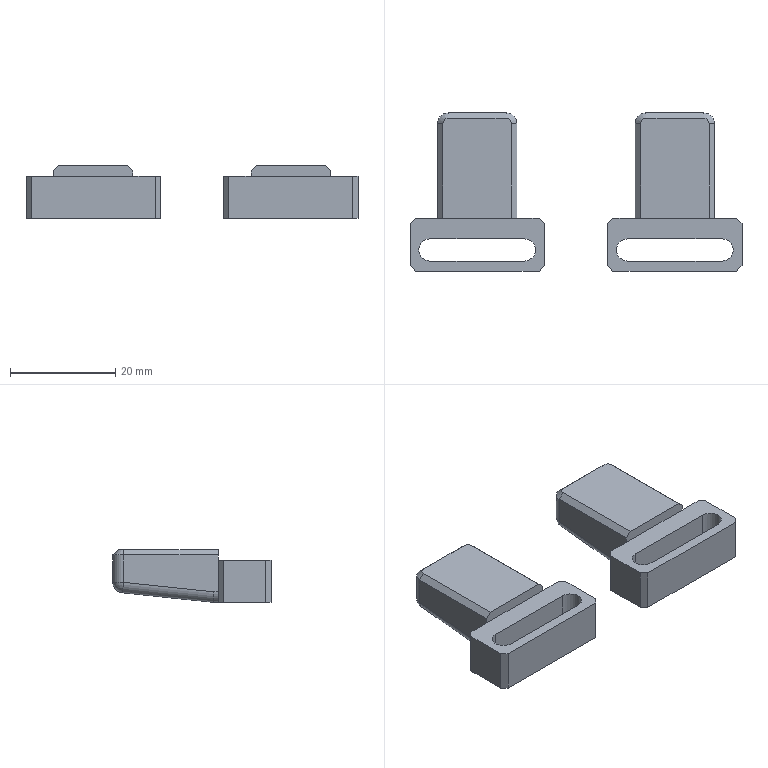NC program | NX | posted with a generic post | part box 63 x 30 x 10 mm
Lines 1 to 136 of 24780:
N10 G17 G21 G94 G90
(FLOOR_WALL_COPY_COPY , TOOL : D80)
N12 T19 M6
N14 G54
N16 G17 G0 G90 X78.5 Y0. B0. C0. S6500 M3
N18 G43 Z30. H19
N20 Z7.04
N22 G94 G1 Z4.04 F1500.
N24 X73.5
N26 X-73.5
N28 X-78.5
N30 Z7.04
N32 G0 Z30.
N34 X78.5
N36 Z6.08
N38 G1 Z3.08
N40 X73.5
N42 X-73.5
N44 X-78.5
N46 Z6.08
N48 G0 Z30.
N50 X78.5
N52 Z5.12
N54 G1 Z2.12
N56 X73.5
N58 X-73.5
N60 X-78.5
N62 Z5.12
N64 G0 Z30.
N66 X78.5
N68 Z4.16
N70 G1 Z1.16
N72 X73.5
N74 X-73.5
N76 X-78.5
N78 Z4.16
N80 G0 Z30.
N82 X78.5
N84 Z3.2
N86 G1 Z0.2
N88 X73.5
N90 X-73.5
N92 X-78.5
N94 Z3.2
N96 G0 Z30.
(FLOOR_WALL_COPY_COPY_COPY , TOOL : D80)
N98 X78.5
N100 Z3.
N102 G1 Z0.
N104 X73.5
N106 X-73.5
N108 X-78.5
N110 Z3.
N112 G0 Z30.
N114 M5
(PLANAR_MILL_COPY_COPY_COPY_COPY_COPY_COPY_1_COPY_1_COPY_1 , TOOL : D6A45)
N116 T01 M6
N118 G54
N120 G17 G0 G90 X-17.48 Y11. B0. C0. S9500 M3
N122 G43 Z30. H1
N124 Z0.5
N126 G94 G1 Z-1. F1250.
N128 X-17.884 Y11.7
N130 G3 X-18.75 Y12.2 R1.
N132 G1 X-27.75
N134 G3 X-28.95 Y11. R1.2
N136 X-27.75 Y9.8 R1.2
N138 G1 X-9.75
N140 G3 X-8.55 Y11. R1.2
N142 X-9.75 Y12.2 R1.2
N144 G1 X-18.75
N146 G3 X-19.616 Y11.7 R1.
N148 G1 X-20.02 Y11.
N150 Z0.5
N152 G0 Z30.
N154 X-33.962 Y7.378
N156 Z0.5
N158 G1 Z-1.
N160 X-33.387 Y7.16
N162 G3 X-32.4 Y7.322 R1.
N164 G1 Y13.959
N166 G2 X-32.107 Y14.666 R1.
N168 G1 X-31.166 Y15.607
N170 G2 X-30.459 Y15.9 R1.
N172 G1 X-7.041
N174 G2 X-6.334 Y15.607 R1.
N176 G1 X-5.393 Y14.666
N178 G2 X-5.1 Y13.959 R1.
N180 G1 Y8.
N182 G3 X-4.234 Y8.5 R1.
N184 G1 X-3.83 Y9.2
N186 Z0.5
N188 G0 Z30.
N190 X3.83
N192 Z0.5
N194 G1 Z-1.
N196 X4.234 Y8.5
N198 G3 X5.1 Y8. R1.
N200 G1 Y13.959
N202 G2 X5.393 Y14.666 R1.
N204 G1 X6.334 Y15.607
N206 G2 X7.041 Y15.9 R1.
N208 G1 X30.459
N210 G2 X31.166 Y15.607 R1.
N212 G1 X32.107 Y14.666
N214 G2 X32.4 Y13.959 R1.
N216 G1 Y7.322
N218 G3 X33.387 Y7.16 R1.
N220 G1 X33.962 Y7.378
N222 Z0.5
N224 G0 Z30.
N226 X20.02 Y11.
N228 Z0.5
N230 G1 Z-1.
N232 X19.616 Y11.7
N234 G3 X18.75 Y12.2 R1.
N236 G1 X9.75
N238 G3 X8.55 Y11. R1.2
N240 X9.75 Y9.8 R1.2
N242 G1 X27.75
N244 G3 X28.95 Y11. R1.2
N246 X27.75 Y12.2 R1.2
N248 G1 X18.75
N250 G3 X17.884 Y11.7 R1.
N252 G1 X17.48 Y11.
N254 Z0.5
N256 G0 Z30.
N258 M5